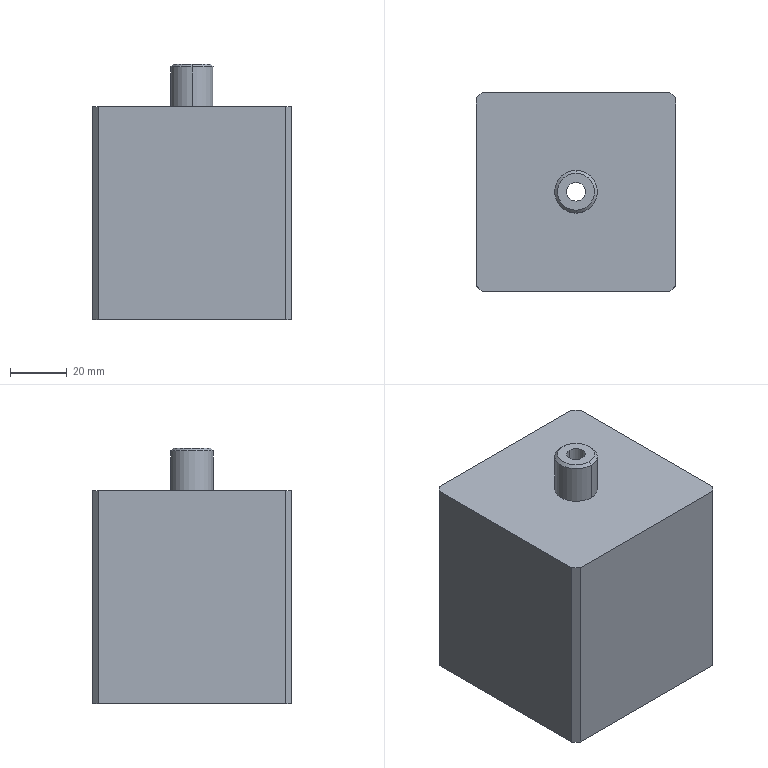NC program | NX | posted with a generic post | part box 70 x 70 x 90 mm
Lines 1 to 1715 of 2643, first 1589 of 1703 lines:
N10 G17 G21 G94 G90
(FLOOR_WALL , TOOL : D63)
N12 T01 M6
N14 G54
N16 G17 G0 G90 X-72.5 Y37.997 S6500 M3
N18 G43 Z30. H1
N20 Z3.
N22 G94 G1 Z0. F2500.
N24 X-69.5
N26 X69.5
N28 Y12.599
N30 X-69.5
N32 Y-12.8
N34 X69.5
N36 X72.5
N38 Z3.
N40 G0 Z30.
N42 M5
(DRILLING , TOOL : D8A45)
N44 T06 M6
N46 G54
N48 G17 G0 G90 X0. Y0. S5000 M3
N50 G43 Z30. H6
N52 G94 G81 G98 Z-3.4 F250. R3.
N54 G80
N56 G0 X0. Y0. Z30.
N58 M5
(DRILLING_COPY , TOOL : 6.6ZT)
N60 T16 M6
N62 G54
N64 G17 G0 G90 X0. Y0. S2000 M3
N66 G43 Z30. H16
N68 G94 G83 G98 Z-26.983 F250. Q2. R3.
N70 G80
N72 G0 X0. Y0. Z30.
N74 M5
(ZLEVEL_PROFILE , TOOL : D16)
N76 T22 M6
N78 G54
N80 G17 G0 G90 X-2.862 Y-43.15 S7500 M3
N82 G43 Z30. H22
N84 Z1.4
N86 G94 G1 X-33. Z-0.179 F1000.
N88 X-33.7 Z-0.216
N90 X-35.342 Y-42.838 Z-0.304
N92 X-36.886 Y-42.198 Z-0.391
N94 X-38.268 Y-41.258 Z-0.479
N96 X-41.258 Y-38.268 Z-0.701
N98 X-42.198 Y-36.886 Z-0.788
N100 X-42.838 Y-35.342 Z-0.876
N102 X-43.15 Y-33.7 Z-0.963
N104 Y-33. Z-1.
N106 Y33. F2500.
N108 G2 X-40.763 Y38.763 R8.15
N110 G1 X-38.763 Y40.763
N112 G2 X-33. Y43.15 R8.15
N114 G1 X33.
N116 G2 X38.763 Y40.763 R8.15
N118 G1 X40.763 Y38.763
N120 G2 X43.15 Y33. R8.15
N122 G1 Y-33.
N124 G2 X40.763 Y-38.763 R8.15
N126 G1 X38.763 Y-40.763
N128 G2 X33. Y-43.15 R8.15
N130 G1 X-33.
N132 G2 X-38.763 Y-40.763 R8.15
N134 G1 X-40.763 Y-38.763
N136 G2 X-43.15 Y-33. R8.15
N138 G1 Y24.29 Z-2.
N140 Y33.
N142 G2 X-40.763 Y38.763 R8.15
N144 G1 X-38.763 Y40.763
N146 G2 X-33. Y43.15 R8.15
N148 G1 X33.
N150 G2 X38.763 Y40.763 R8.15
N152 G1 X40.763 Y38.763
N154 G2 X43.15 Y33. R8.15
N156 G1 Y-33.
N158 G2 X40.763 Y-38.763 R8.15
N160 G1 X38.763 Y-40.763
N162 G2 X33. Y-43.15 R8.15
N164 G1 X-33.
N166 G2 X-38.763 Y-40.763 R8.15
N168 G1 X-40.763 Y-38.763
N170 G2 X-43.15 Y-33. R8.15
N172 G1 Y24.29 Z-3.
N174 Y33.
N176 G2 X-40.763 Y38.763 R8.15
N178 G1 X-38.763 Y40.763
N180 G2 X-33. Y43.15 R8.15
N182 G1 X33.
N184 G2 X38.763 Y40.763 R8.15
N186 G1 X40.763 Y38.763
N188 G2 X43.15 Y33. R8.15
N190 G1 Y-33.
N192 G2 X40.763 Y-38.763 R8.15
N194 G1 X38.763 Y-40.763
N196 G2 X33. Y-43.15 R8.15
N198 G1 X-33.
N200 G2 X-38.763 Y-40.763 R8.15
N202 G1 X-40.763 Y-38.763
N204 G2 X-43.15 Y-33. R8.15
N206 G1 Y24.29 Z-4.
N208 Y33.
N210 G2 X-40.763 Y38.763 R8.15
N212 G1 X-38.763 Y40.763
N214 G2 X-33. Y43.15 R8.15
N216 G1 X33.
N218 G2 X38.763 Y40.763 R8.15
N220 G1 X40.763 Y38.763
N222 G2 X43.15 Y33. R8.15
N224 G1 Y-33.
N226 G2 X40.763 Y-38.763 R8.15
N228 G1 X38.763 Y-40.763
N230 G2 X33. Y-43.15 R8.15
N232 G1 X-33.
N234 G2 X-38.763 Y-40.763 R8.15
N236 G1 X-40.763 Y-38.763
N238 G2 X-43.15 Y-33. R8.15
N240 G1 Y24.29 Z-5.
N242 Y33.
N244 G2 X-40.763 Y38.763 R8.15
N246 G1 X-38.763 Y40.763
N248 G2 X-33. Y43.15 R8.15
N250 G1 X33.
N252 G2 X38.763 Y40.763 R8.15
N254 G1 X40.763 Y38.763
N256 G2 X43.15 Y33. R8.15
N258 G1 Y-33.
N260 G2 X40.763 Y-38.763 R8.15
N262 G1 X38.763 Y-40.763
N264 G2 X33. Y-43.15 R8.15
N266 G1 X-33.
N268 G2 X-38.763 Y-40.763 R8.15
N270 G1 X-40.763 Y-38.763
N272 G2 X-43.15 Y-33. R8.15
N274 G1 Y24.29 Z-6.
N276 Y33.
N278 G2 X-40.763 Y38.763 R8.15
N280 G1 X-38.763 Y40.763
N282 G2 X-33. Y43.15 R8.15
N284 G1 X33.
N286 G2 X38.763 Y40.763 R8.15
N288 G1 X40.763 Y38.763
N290 G2 X43.15 Y33. R8.15
N292 G1 Y-33.
N294 G2 X40.763 Y-38.763 R8.15
N296 G1 X38.763 Y-40.763
N298 G2 X33. Y-43.15 R8.15
N300 G1 X-33.
N302 G2 X-38.763 Y-40.763 R8.15
N304 G1 X-40.763 Y-38.763
N306 G2 X-43.15 Y-33. R8.15
N308 G1 Y24.29 Z-7.
N310 Y33.
N312 G2 X-40.763 Y38.763 R8.15
N314 G1 X-38.763 Y40.763
N316 G2 X-33. Y43.15 R8.15
N318 G1 X33.
N320 G2 X38.763 Y40.763 R8.15
N322 G1 X40.763 Y38.763
N324 G2 X43.15 Y33. R8.15
N326 G1 Y-33.
N328 G2 X40.763 Y-38.763 R8.15
N330 G1 X38.763 Y-40.763
N332 G2 X33. Y-43.15 R8.15
N334 G1 X-33.
N336 G2 X-38.763 Y-40.763 R8.15
N338 G1 X-40.763 Y-38.763
N340 G2 X-43.15 Y-33. R8.15
N342 G1 Y24.29 Z-8.
N344 Y33.
N346 G2 X-40.763 Y38.763 R8.15
N348 G1 X-38.763 Y40.763
N350 G2 X-33. Y43.15 R8.15
N352 G1 X33.
N354 G2 X38.763 Y40.763 R8.15
N356 G1 X40.763 Y38.763
N358 G2 X43.15 Y33. R8.15
N360 G1 Y-33.
N362 G2 X40.763 Y-38.763 R8.15
N364 G1 X38.763 Y-40.763
N366 G2 X33. Y-43.15 R8.15
N368 G1 X-33.
N370 G2 X-38.763 Y-40.763 R8.15
N372 G1 X-40.763 Y-38.763
N374 G2 X-43.15 Y-33. R8.15
N376 G1 Y24.29 Z-9.
N378 Y33.
N380 G2 X-40.763 Y38.763 R8.15
N382 G1 X-38.763 Y40.763
N384 G2 X-33. Y43.15 R8.15
N386 G1 X33.
N388 G2 X38.763 Y40.763 R8.15
N390 G1 X40.763 Y38.763
N392 G2 X43.15 Y33. R8.15
N394 G1 Y-33.
N396 G2 X40.763 Y-38.763 R8.15
N398 G1 X38.763 Y-40.763
N400 G2 X33. Y-43.15 R8.15
N402 G1 X-33.
N404 G2 X-38.763 Y-40.763 R8.15
N406 G1 X-40.763 Y-38.763
N408 G2 X-43.15 Y-33. R8.15
N410 G1 Y24.29 Z-10.
N412 Y33.
N414 G2 X-40.763 Y38.763 R8.15
N416 G1 X-38.763 Y40.763
N418 G2 X-33. Y43.15 R8.15
N420 G1 X33.
N422 G2 X38.763 Y40.763 R8.15
N424 G1 X40.763 Y38.763
N426 G2 X43.15 Y33. R8.15
N428 G1 Y-33.
N430 G2 X40.763 Y-38.763 R8.15
N432 G1 X38.763 Y-40.763
N434 G2 X33. Y-43.15 R8.15
N436 G1 X-33.
N438 G2 X-38.763 Y-40.763 R8.15
N440 G1 X-40.763 Y-38.763
N442 G2 X-43.15 Y-33. R8.15
N444 G1 Y24.29 Z-11.
N446 Y33.
N448 G2 X-40.763 Y38.763 R8.15
N450 G1 X-38.763 Y40.763
N452 G2 X-33. Y43.15 R8.15
N454 G1 X33.
N456 G2 X38.763 Y40.763 R8.15
N458 G1 X40.763 Y38.763
N460 G2 X43.15 Y33. R8.15
N462 G1 Y-33.
N464 G2 X40.763 Y-38.763 R8.15
N466 G1 X38.763 Y-40.763
N468 G2 X33. Y-43.15 R8.15
N470 G1 X-33.
N472 G2 X-38.763 Y-40.763 R8.15
N474 G1 X-40.763 Y-38.763
N476 G2 X-43.15 Y-33. R8.15
N478 G1 Y24.29 Z-12.
N480 Y33.
N482 G2 X-40.763 Y38.763 R8.15
N484 G1 X-38.763 Y40.763
N486 G2 X-33. Y43.15 R8.15
N488 G1 X33.
N490 G2 X38.763 Y40.763 R8.15
N492 G1 X40.763 Y38.763
N494 G2 X43.15 Y33. R8.15
N496 G1 Y-33.
N498 G2 X40.763 Y-38.763 R8.15
N500 G1 X38.763 Y-40.763
N502 G2 X33. Y-43.15 R8.15
N504 G1 X-33.
N506 G2 X-38.763 Y-40.763 R8.15
N508 G1 X-40.763 Y-38.763
N510 G2 X-43.15 Y-33. R8.15
N512 G1 Y24.29 Z-13.
N514 Y33.
N516 G2 X-40.763 Y38.763 R8.15
N518 G1 X-38.763 Y40.763
N520 G2 X-33. Y43.15 R8.15
N522 G1 X33.
N524 G2 X38.763 Y40.763 R8.15
N526 G1 X40.763 Y38.763
N528 G2 X43.15 Y33. R8.15
N530 G1 Y-33.
N532 G2 X40.763 Y-38.763 R8.15
N534 G1 X38.763 Y-40.763
N536 G2 X33. Y-43.15 R8.15
N538 G1 X-33.
N540 G2 X-38.763 Y-40.763 R8.15
N542 G1 X-40.763 Y-38.763
N544 G2 X-43.15 Y-33. R8.15
N546 G1 Y24.29 Z-14.
N548 Y33.
N550 G2 X-40.763 Y38.763 R8.15
N552 G1 X-38.763 Y40.763
N554 G2 X-33. Y43.15 R8.15
N556 G1 X33.
N558 G2 X38.763 Y40.763 R8.15
N560 G1 X40.763 Y38.763
N562 G2 X43.15 Y33. R8.15
N564 G1 Y-33.
N566 G2 X40.763 Y-38.763 R8.15
N568 G1 X38.763 Y-40.763
N570 G2 X33. Y-43.15 R8.15
N572 G1 X-33.
N574 G2 X-38.763 Y-40.763 R8.15
N576 G1 X-40.763 Y-38.763
N578 G2 X-43.15 Y-33. R8.15
N580 G1 Y24.29 Z-15.
N582 Y33.
N584 G2 X-40.763 Y38.763 R8.15
N586 G1 X-38.763 Y40.763
N588 G2 X-33. Y43.15 R8.15
N590 G1 X33.
N592 G2 X38.763 Y40.763 R8.15
N594 G1 X40.763 Y38.763
N596 G2 X43.15 Y33. R8.15
N598 G1 Y-33.
N600 G2 X40.763 Y-38.763 R8.15
N602 G1 X38.763 Y-40.763
N604 G2 X33. Y-43.15 R8.15
N606 G1 X-33.
N608 G2 X-38.763 Y-40.763 R8.15
N610 G1 X-40.763 Y-38.763
N612 G2 X-43.15 Y-33. R8.15
N614 G1 Y24.29 Z-16.
N616 Y33.
N618 G2 X-40.763 Y38.763 R8.15
N620 G1 X-38.763 Y40.763
N622 G2 X-33. Y43.15 R8.15
N624 G1 X33.
N626 G2 X38.763 Y40.763 R8.15
N628 G1 X40.763 Y38.763
N630 G2 X43.15 Y33. R8.15
N632 G1 Y-33.
N634 G2 X40.763 Y-38.763 R8.15
N636 G1 X38.763 Y-40.763
N638 G2 X33. Y-43.15 R8.15
N640 G1 X-33.
N642 G2 X-38.763 Y-40.763 R8.15
N644 G1 X-40.763 Y-38.763
N646 G2 X-43.15 Y-33. R8.15
N648 G1 Y24.29 Z-17.
N650 Y33.
N652 G2 X-40.763 Y38.763 R8.15
N654 G1 X-38.763 Y40.763
N656 G2 X-33. Y43.15 R8.15
N658 G1 X33.
N660 G2 X38.763 Y40.763 R8.15
N662 G1 X40.763 Y38.763
N664 G2 X43.15 Y33. R8.15
N666 G1 Y-33.
N668 G2 X40.763 Y-38.763 R8.15
N670 G1 X38.763 Y-40.763
N672 G2 X33. Y-43.15 R8.15
N674 G1 X-33.
N676 G2 X-38.763 Y-40.763 R8.15
N678 G1 X-40.763 Y-38.763
N680 G2 X-43.15 Y-33. R8.15
N682 G1 Y24.29 Z-18.
N684 Y33.
N686 G2 X-40.763 Y38.763 R8.15
N688 G1 X-38.763 Y40.763
N690 G2 X-33. Y43.15 R8.15
N692 G1 X33.
N694 G2 X38.763 Y40.763 R8.15
N696 G1 X40.763 Y38.763
N698 G2 X43.15 Y33. R8.15
N700 G1 Y-33.
N702 G2 X40.763 Y-38.763 R8.15
N704 G1 X38.763 Y-40.763
N706 G2 X33. Y-43.15 R8.15
N708 G1 X-33.
N710 G2 X-38.763 Y-40.763 R8.15
N712 G1 X-40.763 Y-38.763
N714 G2 X-43.15 Y-33. R8.15
N716 G1 Y24.29 Z-19.
N718 Y33.
N720 G2 X-40.763 Y38.763 R8.15
N722 G1 X-38.763 Y40.763
N724 G2 X-33. Y43.15 R8.15
N726 G1 X33.
N728 G2 X38.763 Y40.763 R8.15
N730 G1 X40.763 Y38.763
N732 G2 X43.15 Y33. R8.15
N734 G1 Y-33.
N736 G2 X40.763 Y-38.763 R8.15
N738 G1 X38.763 Y-40.763
N740 G2 X33. Y-43.15 R8.15
N742 G1 X-33.
N744 G2 X-38.763 Y-40.763 R8.15
N746 G1 X-40.763 Y-38.763
N748 G2 X-43.15 Y-33. R8.15
N750 G1 Y24.29 Z-20.
N752 Y33.
N754 G2 X-40.763 Y38.763 R8.15
N756 G1 X-38.763 Y40.763
N758 G2 X-33. Y43.15 R8.15
N760 G1 X33.
N762 G2 X38.763 Y40.763 R8.15
N764 G1 X40.763 Y38.763
N766 G2 X43.15 Y33. R8.15
N768 G1 Y-33.
N770 G2 X40.763 Y-38.763 R8.15
N772 G1 X38.763 Y-40.763
N774 G2 X33. Y-43.15 R8.15
N776 G1 X-33.
N778 G2 X-38.763 Y-40.763 R8.15
N780 G1 X-40.763 Y-38.763
N782 G2 X-43.15 Y-33. R8.15
N784 G1 Y24.29 Z-21.
N786 Y33.
N788 G2 X-40.763 Y38.763 R8.15
N790 G1 X-38.763 Y40.763
N792 G2 X-33. Y43.15 R8.15
N794 G1 X33.
N796 G2 X38.763 Y40.763 R8.15
N798 G1 X40.763 Y38.763
N800 G2 X43.15 Y33. R8.15
N802 G1 Y-33.
N804 G2 X40.763 Y-38.763 R8.15
N806 G1 X38.763 Y-40.763
N808 G2 X33. Y-43.15 R8.15
N810 G1 X-33.
N812 G2 X-38.763 Y-40.763 R8.15
N814 G1 X-40.763 Y-38.763
N816 G2 X-43.15 Y-33. R8.15
N818 G1 Y24.29 Z-22.
N820 Y33.
N822 G2 X-40.763 Y38.763 R8.15
N824 G1 X-38.763 Y40.763
N826 G2 X-33. Y43.15 R8.15
N828 G1 X33.
N830 G2 X38.763 Y40.763 R8.15
N832 G1 X40.763 Y38.763
N834 G2 X43.15 Y33. R8.15
N836 G1 Y-33.
N838 G2 X40.763 Y-38.763 R8.15
N840 G1 X38.763 Y-40.763
N842 G2 X33. Y-43.15 R8.15
N844 G1 X-33.
N846 G2 X-38.763 Y-40.763 R8.15
N848 G1 X-40.763 Y-38.763
N850 G2 X-43.15 Y-33. R8.15
N852 G1 Y24.29 Z-23.
N854 Y33.
N856 G2 X-40.763 Y38.763 R8.15
N858 G1 X-38.763 Y40.763
N860 G2 X-33. Y43.15 R8.15
N862 G1 X33.
N864 G2 X38.763 Y40.763 R8.15
N866 G1 X40.763 Y38.763
N868 G2 X43.15 Y33. R8.15
N870 G1 Y-33.
N872 G2 X40.763 Y-38.763 R8.15
N874 G1 X38.763 Y-40.763
N876 G2 X33. Y-43.15 R8.15
N878 G1 X-33.
N880 G2 X-38.763 Y-40.763 R8.15
N882 G1 X-40.763 Y-38.763
N884 G2 X-43.15 Y-33. R8.15
N886 G1 Y24.29 Z-24.
N888 Y33.
N890 G2 X-40.763 Y38.763 R8.15
N892 G1 X-38.763 Y40.763
N894 G2 X-33. Y43.15 R8.15
N896 G1 X33.
N898 G2 X38.763 Y40.763 R8.15
N900 G1 X40.763 Y38.763
N902 G2 X43.15 Y33. R8.15
N904 G1 Y-33.
N906 G2 X40.763 Y-38.763 R8.15
N908 G1 X38.763 Y-40.763
N910 G2 X33. Y-43.15 R8.15
N912 G1 X-33.
N914 G2 X-38.763 Y-40.763 R8.15
N916 G1 X-40.763 Y-38.763
N918 G2 X-43.15 Y-33. R8.15
N920 G1 Y24.29 Z-25.
N922 Y33.
N924 G2 X-40.763 Y38.763 R8.15
N926 G1 X-38.763 Y40.763
N928 G2 X-33. Y43.15 R8.15
N930 G1 X33.
N932 G2 X38.763 Y40.763 R8.15
N934 G1 X40.763 Y38.763
N936 G2 X43.15 Y33. R8.15
N938 G1 Y-33.
N940 G2 X40.763 Y-38.763 R8.15
N942 G1 X38.763 Y-40.763
N944 G2 X33. Y-43.15 R8.15
N946 G1 X-33.
N948 G2 X-38.763 Y-40.763 R8.15
N950 G1 X-40.763 Y-38.763
N952 G2 X-43.15 Y-33. R8.15
N954 G1 Y24.29 Z-26.
N956 Y33.
N958 G2 X-40.763 Y38.763 R8.15
N960 G1 X-38.763 Y40.763
N962 G2 X-33. Y43.15 R8.15
N964 G1 X33.
N966 G2 X38.763 Y40.763 R8.15
N968 G1 X40.763 Y38.763
N970 G2 X43.15 Y33. R8.15
N972 G1 Y-33.
N974 G2 X40.763 Y-38.763 R8.15
N976 G1 X38.763 Y-40.763
N978 G2 X33. Y-43.15 R8.15
N980 G1 X-33.
N982 G2 X-38.763 Y-40.763 R8.15
N984 G1 X-40.763 Y-38.763
N986 G2 X-43.15 Y-33. R8.15
N988 G1 Y24.29 Z-27.
N990 Y33.
N992 G2 X-40.763 Y38.763 R8.15
N994 G1 X-38.763 Y40.763
N996 G2 X-33. Y43.15 R8.15
N998 G1 X33.
N1000 G2 X38.763 Y40.763 R8.15
N1002 G1 X40.763 Y38.763
N1004 G2 X43.15 Y33. R8.15
N1006 G1 Y-33.
N1008 G2 X40.763 Y-38.763 R8.15
N1010 G1 X38.763 Y-40.763
N1012 G2 X33. Y-43.15 R8.15
N1014 G1 X-33.
N1016 G2 X-38.763 Y-40.763 R8.15
N1018 G1 X-40.763 Y-38.763
N1020 G2 X-43.15 Y-33. R8.15
N1022 G1 Y24.29 Z-28.
N1024 Y33.
N1026 G2 X-40.763 Y38.763 R8.15
N1028 G1 X-38.763 Y40.763
N1030 G2 X-33. Y43.15 R8.15
N1032 G1 X33.
N1034 G2 X38.763 Y40.763 R8.15
N1036 G1 X40.763 Y38.763
N1038 G2 X43.15 Y33. R8.15
N1040 G1 Y-33.
N1042 G2 X40.763 Y-38.763 R8.15
N1044 G1 X38.763 Y-40.763
N1046 G2 X33. Y-43.15 R8.15
N1048 G1 X-33.
N1050 G2 X-38.763 Y-40.763 R8.15
N1052 G1 X-40.763 Y-38.763
N1054 G2 X-43.15 Y-33. R8.15
N1056 G1 Y24.29 Z-29.
N1058 Y33.
N1060 G2 X-40.763 Y38.763 R8.15
N1062 G1 X-38.763 Y40.763
N1064 G2 X-33. Y43.15 R8.15
N1066 G1 X33.
N1068 G2 X38.763 Y40.763 R8.15
N1070 G1 X40.763 Y38.763
N1072 G2 X43.15 Y33. R8.15
N1074 G1 Y-33.
N1076 G2 X40.763 Y-38.763 R8.15
N1078 G1 X38.763 Y-40.763
N1080 G2 X33. Y-43.15 R8.15
N1082 G1 X-33.
N1084 G2 X-38.763 Y-40.763 R8.15
N1086 G1 X-40.763 Y-38.763
N1088 G2 X-43.15 Y-33. R8.15
N1090 G1 Y24.29 Z-30.
N1092 Y33.
N1094 G2 X-40.763 Y38.763 R8.15
N1096 G1 X-38.763 Y40.763
N1098 G2 X-33. Y43.15 R8.15
N1100 G1 X33.
N1102 G2 X38.763 Y40.763 R8.15
N1104 G1 X40.763 Y38.763
N1106 G2 X43.15 Y33. R8.15
N1108 G1 Y-33.
N1110 G2 X40.763 Y-38.763 R8.15
N1112 G1 X38.763 Y-40.763
N1114 G2 X33. Y-43.15 R8.15
N1116 G1 X-33.
N1118 G2 X-38.763 Y-40.763 R8.15
N1120 G1 X-40.763 Y-38.763
N1122 G2 X-43.15 Y-33. R8.15
N1124 G1 Y24.29 Z-31.
N1126 Y33.
N1128 G2 X-40.763 Y38.763 R8.15
N1130 G1 X-38.763 Y40.763
N1132 G2 X-33. Y43.15 R8.15
N1134 G1 X33.
N1136 G2 X38.763 Y40.763 R8.15
N1138 G1 X40.763 Y38.763
N1140 G2 X43.15 Y33. R8.15
N1142 G1 Y-33.
N1144 G2 X40.763 Y-38.763 R8.15
N1146 G1 X38.763 Y-40.763
N1148 G2 X33. Y-43.15 R8.15
N1150 G1 X-33.
N1152 G2 X-38.763 Y-40.763 R8.15
N1154 G1 X-40.763 Y-38.763
N1156 G2 X-43.15 Y-33. R8.15
N1158 G1 Y24.29 Z-32.
N1160 Y33.
N1162 G2 X-40.763 Y38.763 R8.15
N1164 G1 X-38.763 Y40.763
N1166 G2 X-33. Y43.15 R8.15
N1168 G1 X33.
N1170 G2 X38.763 Y40.763 R8.15
N1172 G1 X40.763 Y38.763
N1174 G2 X43.15 Y33. R8.15
N1176 G1 Y-33.
N1178 G2 X40.763 Y-38.763 R8.15
N1180 G1 X38.763 Y-40.763
N1182 G2 X33. Y-43.15 R8.15
N1184 G1 X-33.
N1186 G2 X-38.763 Y-40.763 R8.15
N1188 G1 X-40.763 Y-38.763
N1190 G2 X-43.15 Y-33. R8.15
N1192 G1 Y24.29 Z-33.
N1194 Y33.
N1196 G2 X-40.763 Y38.763 R8.15
N1198 G1 X-38.763 Y40.763
N1200 G2 X-33. Y43.15 R8.15
N1202 G1 X33.
N1204 G2 X38.763 Y40.763 R8.15
N1206 G1 X40.763 Y38.763
N1208 G2 X43.15 Y33. R8.15
N1210 G1 Y-33.
N1212 G2 X40.763 Y-38.763 R8.15
N1214 G1 X38.763 Y-40.763
N1216 G2 X33. Y-43.15 R8.15
N1218 G1 X-33.
N1220 G2 X-38.763 Y-40.763 R8.15
N1222 G1 X-40.763 Y-38.763
N1224 G2 X-43.15 Y-33. R8.15
N1226 G1 Y24.29 Z-34.
N1228 Y33.
N1230 G2 X-40.763 Y38.763 R8.15
N1232 G1 X-38.763 Y40.763
N1234 G2 X-33. Y43.15 R8.15
N1236 G1 X33.
N1238 G2 X38.763 Y40.763 R8.15
N1240 G1 X40.763 Y38.763
N1242 G2 X43.15 Y33. R8.15
N1244 G1 Y-33.
N1246 G2 X40.763 Y-38.763 R8.15
N1248 G1 X38.763 Y-40.763
N1250 G2 X33. Y-43.15 R8.15
N1252 G1 X-33.
N1254 G2 X-38.763 Y-40.763 R8.15
N1256 G1 X-40.763 Y-38.763
N1258 G2 X-43.15 Y-33. R8.15
N1260 G1 Y24.29 Z-35.
N1262 Y33.
N1264 G2 X-40.763 Y38.763 R8.15
N1266 G1 X-38.763 Y40.763
N1268 G2 X-33. Y43.15 R8.15
N1270 G1 X33.
N1272 G2 X38.763 Y40.763 R8.15
N1274 G1 X40.763 Y38.763
N1276 G2 X43.15 Y33. R8.15
N1278 G1 Y-33.
N1280 G2 X40.763 Y-38.763 R8.15
N1282 G1 X38.763 Y-40.763
N1284 G2 X33. Y-43.15 R8.15
N1286 G1 X-33.
N1288 G2 X-38.763 Y-40.763 R8.15
N1290 G1 X-40.763 Y-38.763
N1292 G2 X-43.15 Y-33. R8.15
N1294 G1 Y24.29 Z-36.
N1296 Y33.
N1298 G2 X-40.763 Y38.763 R8.15
N1300 G1 X-38.763 Y40.763
N1302 G2 X-33. Y43.15 R8.15
N1304 G1 X33.
N1306 G2 X38.763 Y40.763 R8.15
N1308 G1 X40.763 Y38.763
N1310 G2 X43.15 Y33. R8.15
N1312 G1 Y-33.
N1314 G2 X40.763 Y-38.763 R8.15
N1316 G1 X38.763 Y-40.763
N1318 G2 X33. Y-43.15 R8.15
N1320 G1 X-33.
N1322 G2 X-38.763 Y-40.763 R8.15
N1324 G1 X-40.763 Y-38.763
N1326 G2 X-43.15 Y-33. R8.15
N1328 G1 Y24.29 Z-37.
N1330 Y33.
N1332 G2 X-40.763 Y38.763 R8.15
N1334 G1 X-38.763 Y40.763
N1336 G2 X-33. Y43.15 R8.15
N1338 G1 X33.
N1340 G2 X38.763 Y40.763 R8.15
N1342 G1 X40.763 Y38.763
N1344 G2 X43.15 Y33. R8.15
N1346 G1 Y-33.
N1348 G2 X40.763 Y-38.763 R8.15
N1350 G1 X38.763 Y-40.763
N1352 G2 X33. Y-43.15 R8.15
N1354 G1 X-33.
N1356 G2 X-38.763 Y-40.763 R8.15
N1358 G1 X-40.763 Y-38.763
N1360 G2 X-43.15 Y-33. R8.15
N1362 G1 Y24.29 Z-38.
N1364 Y33.
N1366 G2 X-40.763 Y38.763 R8.15
N1368 G1 X-38.763 Y40.763
N1370 G2 X-33. Y43.15 R8.15
N1372 G1 X33.
N1374 G2 X38.763 Y40.763 R8.15
N1376 G1 X40.763 Y38.763
N1378 G2 X43.15 Y33. R8.15
N1380 G1 Y-33.
N1382 G2 X40.763 Y-38.763 R8.15
N1384 G1 X38.763 Y-40.763
N1386 G2 X33. Y-43.15 R8.15
N1388 G1 X-33.
N1390 G2 X-38.763 Y-40.763 R8.15
N1392 G1 X-40.763 Y-38.763
N1394 G2 X-43.15 Y-33. R8.15
N1396 G1 Y24.29 Z-39.
N1398 Y33.
N1400 G2 X-40.763 Y38.763 R8.15
N1402 G1 X-38.763 Y40.763
N1404 G2 X-33. Y43.15 R8.15
N1406 G1 X33.
N1408 G2 X38.763 Y40.763 R8.15
N1410 G1 X40.763 Y38.763
N1412 G2 X43.15 Y33. R8.15
N1414 G1 Y-33.
N1416 G2 X40.763 Y-38.763 R8.15
N1418 G1 X38.763 Y-40.763
N1420 G2 X33. Y-43.15 R8.15
N1422 G1 X-33.
N1424 G2 X-38.763 Y-40.763 R8.15
N1426 G1 X-40.763 Y-38.763
N1428 G2 X-43.15 Y-33. R8.15
N1430 G1 Y24.29 Z-40.
N1432 Y33.
N1434 G2 X-40.763 Y38.763 R8.15
N1436 G1 X-38.763 Y40.763
N1438 G2 X-33. Y43.15 R8.15
N1440 G1 X33.
N1442 G2 X38.763 Y40.763 R8.15
N1444 G1 X40.763 Y38.763
N1446 G2 X43.15 Y33. R8.15
N1448 G1 Y-33.
N1450 G2 X40.763 Y-38.763 R8.15
N1452 G1 X38.763 Y-40.763
N1454 G2 X33. Y-43.15 R8.15
N1456 G1 X-33.
N1458 G2 X-38.763 Y-40.763 R8.15
N1460 G1 X-40.763 Y-38.763
N1462 G2 X-43.15 Y-33. R8.15
N1464 G1 Y24.29 Z-41.
N1466 Y33.
N1468 G2 X-40.763 Y38.763 R8.15
N1470 G1 X-38.763 Y40.763
N1472 G2 X-33. Y43.15 R8.15
N1474 G1 X33.
N1476 G2 X38.763 Y40.763 R8.15
N1478 G1 X40.763 Y38.763
N1480 G2 X43.15 Y33. R8.15
N1482 G1 Y-33.
N1484 G2 X40.763 Y-38.763 R8.15
N1486 G1 X38.763 Y-40.763
N1488 G2 X33. Y-43.15 R8.15
N1490 G1 X-33.
N1492 G2 X-38.763 Y-40.763 R8.15
N1494 G1 X-40.763 Y-38.763
N1496 G2 X-43.15 Y-33. R8.15
N1498 G1 Y24.29 Z-42.
N1500 Y33.
N1502 G2 X-40.763 Y38.763 R8.15
N1504 G1 X-38.763 Y40.763
N1506 G2 X-33. Y43.15 R8.15
N1508 G1 X33.
N1510 G2 X38.763 Y40.763 R8.15
N1512 G1 X40.763 Y38.763
N1514 G2 X43.15 Y33. R8.15
N1516 G1 Y-33.
N1518 G2 X40.763 Y-38.763 R8.15
N1520 G1 X38.763 Y-40.763
N1522 G2 X33. Y-43.15 R8.15
N1524 G1 X-33.
N1526 G2 X-38.763 Y-40.763 R8.15
N1528 G1 X-40.763 Y-38.763
N1530 G2 X-43.15 Y-33. R8.15
N1532 G1 Y24.29 Z-43.
N1534 Y33.
N1536 G2 X-40.763 Y38.763 R8.15
N1538 G1 X-38.763 Y40.763
N1540 G2 X-33. Y43.15 R8.15
N1542 G1 X33.
N1544 G2 X38.763 Y40.763 R8.15
N1546 G1 X40.763 Y38.763
N1548 G2 X43.15 Y33. R8.15
N1550 G1 Y-33.
N1552 G2 X40.763 Y-38.763 R8.15
N1554 G1 X38.763 Y-40.763
N1556 G2 X33. Y-43.15 R8.15
N1558 G1 X-33.
N1560 G2 X-38.763 Y-40.763 R8.15
N1562 G1 X-40.763 Y-38.763
N1564 G2 X-43.15 Y-33. R8.15
N1566 G1 Y24.29 Z-44.
N1568 Y33.
N1570 G2 X-40.763 Y38.763 R8.15
N1572 G1 X-38.763 Y40.763
N1574 G2 X-33. Y43.15 R8.15
N1576 G1 X33.
N1578 G2 X38.763 Y40.763 R8.15
N1580 G1 X40.763 Y38.763
N1582 G2 X43.15 Y33. R8.15
N1584 G1 Y-33.
N1586 G2 X40.763 Y-38.763 R8.15
N1588 G1 X38.763 Y-40.763
N1590 G2 X33. Y-43.15 R8.15
N1592 G1 X-33.
N1594 G2 X-38.763 Y-40.763 R8.15
N1596 G1 X-40.763 Y-38.763
N1598 G2 X-43.15 Y-33. R8.15
N1600 G1 Y24.29 Z-45.
N1602 Y33.
N1604 G2 X-40.763 Y38.763 R8.15
N1606 G1 X-38.763 Y40.763
N1608 G2 X-33. Y43.15 R8.15
N1610 G1 X33.
N1612 G2 X38.763 Y40.763 R8.15
N1614 G1 X40.763 Y38.763
N1616 G2 X43.15 Y33. R8.15
N1618 G1 Y-33.
N1620 G2 X40.763 Y-38.763 R8.15
N1622 G1 X38.763 Y-40.763
N1624 G2 X33. Y-43.15 R8.15
N1626 G1 X-33.
N1628 G2 X-38.763 Y-40.763 R8.15
N1630 G1 X-40.763 Y-38.763
N1632 G2 X-43.15 Y-33. R8.15
N1634 G1 Y24.29 Z-46.
N1636 Y33.
N1638 G2 X-40.763 Y38.763 R8.15
N1640 G1 X-38.763 Y40.763
N1642 G2 X-33. Y43.15 R8.15
N1644 G1 X33.
N1646 G2 X38.763 Y40.763 R8.15
N1648 G1 X40.763 Y38.763
N1650 G2 X43.15 Y33. R8.15
N1652 G1 Y-33.
N1654 G2 X40.763 Y-38.763 R8.15
N1656 G1 X38.763 Y-40.763
N1658 G2 X33. Y-43.15 R8.15
N1660 G1 X-33.
N1662 G2 X-38.763 Y-40.763 R8.15
N1664 G1 X-40.763 Y-38.763
N1666 G2 X-43.15 Y-33. R8.15
N1668 G1 Y24.29 Z-47.
N1670 Y33.
N1672 G2 X-40.763 Y38.763 R8.15
N1674 G1 X-38.763 Y40.763
N1676 G2 X-33. Y43.15 R8.15
N1678 G1 X33.
N1680 G2 X38.763 Y40.763 R8.15
N1682 G1 X40.763 Y38.763
N1684 G2 X43.15 Y33. R8.15
N1686 G1 Y-33.
N1688 G2 X40.763 Y-38.763 R8.15
N1690 G1 X38.763 Y-40.763
N1692 G2 X33. Y-43.15 R8.15
N1694 G1 X-33.
N1696 G2 X-38.763 Y-40.763 R8.15
N1698 G1 X-40.763 Y-38.763
N1700 G2 X-43.15 Y-33. R8.15
N1702 G1 Y24.29 Z-48.
N1704 Y33.
N1706 G2 X-40.763 Y38.763 R8.15
N1708 G1 X-38.763 Y40.763
N1710 G2 X-33. Y43.15 R8.15
N1712 G1 X33.
N1714 G2 X38.763 Y40.763 R8.15
N1716 G1 X40.763 Y38.763
N1718 G2 X43.15 Y33. R8.15
N1720 G1 Y-33.
N1722 G2 X40.763 Y-38.763 R8.15
N1724 G1 X38.763 Y-40.763
N1726 G2 X33. Y-43.15 R8.15
N1728 G1 X-33.
N1730 G2 X-38.763 Y-40.763 R8.15
N1732 G1 X-40.763 Y-38.763
N1734 G2 X-43.15 Y-33. R8.15
N1736 G1 Y24.29 Z-49.
N1738 Y33.
N1740 G2 X-40.763 Y38.763 R8.15
N1742 G1 X-38.763 Y40.763
N1744 G2 X-33. Y43.15 R8.15
N1746 G1 X33.
N1748 G2 X38.763 Y40.763 R8.15
N1750 G1 X40.763 Y38.763
N1752 G2 X43.15 Y33. R8.15
N1754 G1 Y-33.
N1756 G2 X40.763 Y-38.763 R8.15
N1758 G1 X38.763 Y-40.763
N1760 G2 X33. Y-43.15 R8.15
N1762 G1 X-33.
N1764 G2 X-38.763 Y-40.763 R8.15
N1766 G1 X-40.763 Y-38.763
N1768 G2 X-43.15 Y-33. R8.15
N1770 G1 Y24.29 Z-50.
N1772 Y33.
N1774 G2 X-40.763 Y38.763 R8.15
N1776 G1 X-38.763 Y40.763
N1778 G2 X-33. Y43.15 R8.15
N1780 G1 X33.
N1782 G2 X38.763 Y40.763 R8.15
N1784 G1 X40.763 Y38.763
N1786 G2 X43.15 Y33. R8.15
N1788 G1 Y-33.
N1790 G2 X40.763 Y-38.763 R8.15
N1792 G1 X38.763 Y-40.763
N1794 G2 X33. Y-43.15 R8.15
N1796 G1 X-33.
N1798 G2 X-38.763 Y-40.763 R8.15
N1800 G1 X-40.763 Y-38.763
N1802 G2 X-43.15 Y-33. R8.15
N1804 G1 Y24.29 Z-51.
N1806 Y33.
N1808 G2 X-40.763 Y38.763 R8.15
N1810 G1 X-38.763 Y40.763
N1812 G2 X-33. Y43.15 R8.15
N1814 G1 X33.
N1816 G2 X38.763 Y40.763 R8.15
N1818 G1 X40.763 Y38.763
N1820 G2 X43.15 Y33. R8.15
N1822 G1 Y-33.
N1824 G2 X40.763 Y-38.763 R8.15
N1826 G1 X38.763 Y-40.763
N1828 G2 X33. Y-43.15 R8.15
N1830 G1 X-33.
N1832 G2 X-38.763 Y-40.763 R8.15
N1834 G1 X-40.763 Y-38.763
N1836 G2 X-43.15 Y-33. R8.15
N1838 G1 Y24.29 Z-52.
N1840 Y33.
N1842 G2 X-40.763 Y38.763 R8.15
N1844 G1 X-38.763 Y40.763
N1846 G2 X-33. Y43.15 R8.15
N1848 G1 X33.
N1850 G2 X38.763 Y40.763 R8.15
N1852 G1 X40.763 Y38.763
N1854 G2 X43.15 Y33. R8.15
N1856 G1 Y-33.
N1858 G2 X40.763 Y-38.763 R8.15
N1860 G1 X38.763 Y-40.763
N1862 G2 X33. Y-43.15 R8.15
N1864 G1 X-33.
N1866 G2 X-38.763 Y-40.763 R8.15
N1868 G1 X-40.763 Y-38.763
N1870 G2 X-43.15 Y-33. R8.15
N1872 G1 Y24.29 Z-53.
N1874 Y33.
N1876 G2 X-40.763 Y38.763 R8.15
N1878 G1 X-38.763 Y40.763
N1880 G2 X-33. Y43.15 R8.15
N1882 G1 X33.
N1884 G2 X38.763 Y40.763 R8.15
N1886 G1 X40.763 Y38.763
N1888 G2 X43.15 Y33. R8.15
N1890 G1 Y-33.
N1892 G2 X40.763 Y-38.763 R8.15
N1894 G1 X38.763 Y-40.763
N1896 G2 X33. Y-43.15 R8.15
N1898 G1 X-33.
N1900 G2 X-38.763 Y-40.763 R8.15
N1902 G1 X-40.763 Y-38.763
N1904 G2 X-43.15 Y-33. R8.15
N1906 G1 Y24.29 Z-54.
N1908 Y33.
N1910 G2 X-40.763 Y38.763 R8.15
N1912 G1 X-38.763 Y40.763
N1914 G2 X-33. Y43.15 R8.15
N1916 G1 X33.
N1918 G2 X38.763 Y40.763 R8.15
N1920 G1 X40.763 Y38.763
N1922 G2 X43.15 Y33. R8.15
N1924 G1 Y-33.
N1926 G2 X40.763 Y-38.763 R8.15
N1928 G1 X38.763 Y-40.763
N1930 G2 X33. Y-43.15 R8.15
N1932 G1 X-33.
N1934 G2 X-38.763 Y-40.763 R8.15
N1936 G1 X-40.763 Y-38.763
N1938 G2 X-43.15 Y-33. R8.15
N1940 G1 Y24.29 Z-55.
N1942 Y33.
N1944 G2 X-40.763 Y38.763 R8.15
N1946 G1 X-38.763 Y40.763
N1948 G2 X-33. Y43.15 R8.15
N1950 G1 X33.
N1952 G2 X38.763 Y40.763 R8.15
N1954 G1 X40.763 Y38.763
N1956 G2 X43.15 Y33. R8.15
N1958 G1 Y-33.
N1960 G2 X40.763 Y-38.763 R8.15
N1962 G1 X38.763 Y-40.763
N1964 G2 X33. Y-43.15 R8.15
N1966 G1 X-33.
N1968 G2 X-38.763 Y-40.763 R8.15
N1970 G1 X-40.763 Y-38.763
N1972 G2 X-43.15 Y-33. R8.15
N1974 G1 Y24.29 Z-56.
N1976 Y33.
N1978 G2 X-40.763 Y38.763 R8.15
N1980 G1 X-38.763 Y40.763
N1982 G2 X-33. Y43.15 R8.15
N1984 G1 X33.
N1986 G2 X38.763 Y40.763 R8.15
N1988 G1 X40.763 Y38.763
N1990 G2 X43.15 Y33. R8.15
N1992 G1 Y-33.
N1994 G2 X40.763 Y-38.763 R8.15
N1996 G1 X38.763 Y-40.763
N1998 G2 X33. Y-43.15 R8.15
N2000 G1 X-33.
N2002 G2 X-38.763 Y-40.763 R8.15
N2004 G1 X-40.763 Y-38.763
N2006 G2 X-43.15 Y-33. R8.15
N2008 G1 Y24.29 Z-57.
N2010 Y33.
N2012 G2 X-40.763 Y38.763 R8.15
N2014 G1 X-38.763 Y40.763
N2016 G2 X-33. Y43.15 R8.15
N2018 G1 X33.
N2020 G2 X38.763 Y40.763 R8.15
N2022 G1 X40.763 Y38.763
N2024 G2 X43.15 Y33. R8.15
N2026 G1 Y-33.
N2028 G2 X40.763 Y-38.763 R8.15
N2030 G1 X38.763 Y-40.763
N2032 G2 X33. Y-43.15 R8.15
N2034 G1 X-33.
N2036 G2 X-38.763 Y-40.763 R8.15
N2038 G1 X-40.763 Y-38.763
N2040 G2 X-43.15 Y-33. R8.15
N2042 G1 Y24.29 Z-58.
N2044 Y33.
N2046 G2 X-40.763 Y38.763 R8.15
N2048 G1 X-38.763 Y40.763
N2050 G2 X-33. Y43.15 R8.15
N2052 G1 X33.
N2054 G2 X38.763 Y40.763 R8.15
N2056 G1 X40.763 Y38.763
N2058 G2 X43.15 Y33. R8.15
N2060 G1 Y-33.
N2062 G2 X40.763 Y-38.763 R8.15
N2064 G1 X38.763 Y-40.763
N2066 G2 X33. Y-43.15 R8.15
N2068 G1 X-33.
N2070 G2 X-38.763 Y-40.763 R8.15
N2072 G1 X-40.763 Y-38.763
N2074 G2 X-43.15 Y-33. R8.15
N2076 G1 Y24.29 Z-59.
N2078 Y33.
N2080 G2 X-40.763 Y38.763 R8.15
N2082 G1 X-38.763 Y40.763
N2084 G2 X-33. Y43.15 R8.15
N2086 G1 X33.
N2088 G2 X38.763 Y40.763 R8.15
N2090 G1 X40.763 Y38.763
N2092 G2 X43.15 Y33. R8.15
N2094 G1 Y-33.
N2096 G2 X40.763 Y-38.763 R8.15
N2098 G1 X38.763 Y-40.763
N2100 G2 X33. Y-43.15 R8.15
N2102 G1 X-33.
N2104 G2 X-38.763 Y-40.763 R8.15
N2106 G1 X-40.763 Y-38.763
N2108 G2 X-43.15 Y-33. R8.15
N2110 G1 Y24.29 Z-60.
N2112 Y33.
N2114 G2 X-40.763 Y38.763 R8.15
N2116 G1 X-38.763 Y40.763
N2118 G2 X-33. Y43.15 R8.15
N2120 G1 X33.
N2122 G2 X38.763 Y40.763 R8.15
N2124 G1 X40.763 Y38.763
N2126 G2 X43.15 Y33. R8.15
N2128 G1 Y-33.
N2130 G2 X40.763 Y-38.763 R8.15
N2132 G1 X38.763 Y-40.763
N2134 G2 X33. Y-43.15 R8.15
N2136 G1 X-33.
N2138 G2 X-38.763 Y-40.763 R8.15
N2140 G1 X-40.763 Y-38.763
N2142 G2 X-43.15 Y-33. R8.15
N2144 G1 Y24.29 Z-61.
N2146 Y33.
N2148 G2 X-40.763 Y38.763 R8.15
N2150 G1 X-38.763 Y40.763
N2152 G2 X-33. Y43.15 R8.15
N2154 G1 X33.
N2156 G2 X38.763 Y40.763 R8.15
N2158 G1 X40.763 Y38.763
N2160 G2 X43.15 Y33. R8.15
N2162 G1 Y-33.
N2164 G2 X40.763 Y-38.763 R8.15
N2166 G1 X38.763 Y-40.763
N2168 G2 X33. Y-43.15 R8.15
N2170 G1 X-33.
N2172 G2 X-38.763 Y-40.763 R8.15
N2174 G1 X-40.763 Y-38.763
N2176 G2 X-43.15 Y-33. R8.15
N2178 G1 Y24.29 Z-62.
N2180 Y33.
N2182 G2 X-40.763 Y38.763 R8.15
N2184 G1 X-38.763 Y40.763
N2186 G2 X-33. Y43.15 R8.15
N2188 G1 X33.
N2190 G2 X38.763 Y40.763 R8.15
N2192 G1 X40.763 Y38.763
N2194 G2 X43.15 Y33. R8.15
N2196 G1 Y-33.
N2198 G2 X40.763 Y-38.763 R8.15
N2200 G1 X38.763 Y-40.763
N2202 G2 X33. Y-43.15 R8.15
N2204 G1 X-33.
N2206 G2 X-38.763 Y-40.763 R8.15
N2208 G1 X-40.763 Y-38.763
N2210 G2 X-43.15 Y-33. R8.15
N2212 G1 Y24.29 Z-63.
N2214 Y33.
N2216 G2 X-40.763 Y38.763 R8.15
N2218 G1 X-38.763 Y40.763
N2220 G2 X-33. Y43.15 R8.15
N2222 G1 X33.
N2224 G2 X38.763 Y40.763 R8.15
N2226 G1 X40.763 Y38.763
N2228 G2 X43.15 Y33. R8.15
N2230 G1 Y-33.
N2232 G2 X40.763 Y-38.763 R8.15
N2234 G1 X38.763 Y-40.763
N2236 G2 X33. Y-43.15 R8.15
N2238 G1 X-33.
N2240 G2 X-38.763 Y-40.763 R8.15
N2242 G1 X-40.763 Y-38.763
N2244 G2 X-43.15 Y-33. R8.15
N2246 G1 Y24.29 Z-64.
N2248 Y33.
N2250 G2 X-40.763 Y38.763 R8.15
N2252 G1 X-38.763 Y40.763
N2254 G2 X-33. Y43.15 R8.15
N2256 G1 X33.
N2258 G2 X38.763 Y40.763 R8.15
N2260 G1 X40.763 Y38.763
N2262 G2 X43.15 Y33. R8.15
N2264 G1 Y-33.
N2266 G2 X40.763 Y-38.763 R8.15
N2268 G1 X38.763 Y-40.763
N2270 G2 X33. Y-43.15 R8.15
N2272 G1 X-33.
N2274 G2 X-38.763 Y-40.763 R8.15
N2276 G1 X-40.763 Y-38.763
N2278 G2 X-43.15 Y-33. R8.15
N2280 G1 Y24.29 Z-65.
N2282 Y33.
N2284 G2 X-40.763 Y38.763 R8.15
N2286 G1 X-38.763 Y40.763
N2288 G2 X-33. Y43.15 R8.15
N2290 G1 X33.
N2292 G2 X38.763 Y40.763 R8.15
N2294 G1 X40.763 Y38.763
N2296 G2 X43.15 Y33. R8.15
N2298 G1 Y-33.
N2300 G2 X40.763 Y-38.763 R8.15
N2302 G1 X38.763 Y-40.763
N2304 G2 X33. Y-43.15 R8.15
N2306 G1 X-33.
N2308 G2 X-38.763 Y-40.763 R8.15
N2310 G1 X-40.763 Y-38.763
N2312 G2 X-43.15 Y-33. R8.15
N2314 G1 Y24.29 Z-66.
N2316 Y33.
N2318 G2 X-40.763 Y38.763 R8.15
N2320 G1 X-38.763 Y40.763
N2322 G2 X-33. Y43.15 R8.15
N2324 G1 X33.
N2326 G2 X38.763 Y40.763 R8.15
N2328 G1 X40.763 Y38.763
N2330 G2 X43.15 Y33. R8.15
N2332 G1 Y-33.
N2334 G2 X40.763 Y-38.763 R8.15
N2336 G1 X38.763 Y-40.763
N2338 G2 X33. Y-43.15 R8.15
N2340 G1 X-33.
N2342 G2 X-38.763 Y-40.763 R8.15
N2344 G1 X-40.763 Y-38.763
N2346 G2 X-43.15 Y-33. R8.15
N2348 G1 Y24.29 Z-67.
N2350 Y33.
N2352 G2 X-40.763 Y38.763 R8.15
N2354 G1 X-38.763 Y40.763
N2356 G2 X-33. Y43.15 R8.15
N2358 G1 X33.
N2360 G2 X38.763 Y40.763 R8.15
N2362 G1 X40.763 Y38.763
N2364 G2 X43.15 Y33. R8.15
N2366 G1 Y-33.
N2368 G2 X40.763 Y-38.763 R8.15
N2370 G1 X38.763 Y-40.763
N2372 G2 X33. Y-43.15 R8.15
N2374 G1 X-33.
N2376 G2 X-38.763 Y-40.763 R8.15
N2378 G1 X-40.763 Y-38.763
N2380 G2 X-43.15 Y-33. R8.15
N2382 G1 Y24.29 Z-68.
N2384 Y33.
N2386 G2 X-40.763 Y38.763 R8.15
N2388 G1 X-38.763 Y40.763
N2390 G2 X-33. Y43.15 R8.15
N2392 G1 X33.
N2394 G2 X38.763 Y40.763 R8.15
N2396 G1 X40.763 Y38.763
N2398 G2 X43.15 Y33. R8.15
N2400 G1 Y-33.
N2402 G2 X40.763 Y-38.763 R8.15
N2404 G1 X38.763 Y-40.763
N2406 G2 X33. Y-43.15 R8.15
N2408 G1 X-33.
N2410 G2 X-38.763 Y-40.763 R8.15
N2412 G1 X-40.763 Y-38.763
N2414 G2 X-43.15 Y-33. R8.15
N2416 G1 Y24.29 Z-69.
N2418 Y33.
N2420 G2 X-40.763 Y38.763 R8.15
N2422 G1 X-38.763 Y40.763
N2424 G2 X-33. Y43.15 R8.15
N2426 G1 X33.
N2428 G2 X38.763 Y40.763 R8.15
N2430 G1 X40.763 Y38.763
N2432 G2 X43.15 Y33. R8.15
N2434 G1 Y-33.
N2436 G2 X40.763 Y-38.763 R8.15
N2438 G1 X38.763 Y-40.763
N2440 G2 X33. Y-43.15 R8.15
N2442 G1 X-33.
N2444 G2 X-38.763 Y-40.763 R8.15
N2446 G1 X-40.763 Y-38.763
N2448 G2 X-43.15 Y-33. R8.15
N2450 G1 Y24.29 Z-70.
N2452 Y33.
N2454 G2 X-40.763 Y38.763 R8.15
N2456 G1 X-38.763 Y40.763
N2458 G2 X-33. Y43.15 R8.15
N2460 G1 X33.
N2462 G2 X38.763 Y40.763 R8.15
N2464 G1 X40.763 Y38.763
N2466 G2 X43.15 Y33. R8.15
N2468 G1 Y-33.
N2470 G2 X40.763 Y-38.763 R8.15
N2472 G1 X38.763 Y-40.763
N2474 G2 X33. Y-43.15 R8.15
N2476 G1 X-33.
N2478 G2 X-38.763 Y-40.763 R8.15
N2480 G1 X-40.763 Y-38.763
N2482 G2 X-43.15 Y-33. R8.15
N2484 G1 Y24.29 Z-71.
N2486 Y33.
N2488 G2 X-40.763 Y38.763 R8.15
N2490 G1 X-38.763 Y40.763
N2492 G2 X-33. Y43.15 R8.15
N2494 G1 X33.
N2496 G2 X38.763 Y40.763 R8.15
N2498 G1 X40.763 Y38.763
N2500 G2 X43.15 Y33. R8.15
N2502 G1 Y-33.
N2504 G2 X40.763 Y-38.763 R8.15
N2506 G1 X38.763 Y-40.763
N2508 G2 X33. Y-43.15 R8.15
N2510 G1 X-33.
N2512 G2 X-38.763 Y-40.763 R8.15
N2514 G1 X-40.763 Y-38.763
N2516 G2 X-43.15 Y-33. R8.15
N2518 G1 Y24.29 Z-72.
N2520 Y33.
N2522 G2 X-40.763 Y38.763 R8.15
N2524 G1 X-38.763 Y40.763
N2526 G2 X-33. Y43.15 R8.15
N2528 G1 X33.
N2530 G2 X38.763 Y40.763 R8.15
N2532 G1 X40.763 Y38.763
N2534 G2 X43.15 Y33. R8.15
N2536 G1 Y-33.
N2538 G2 X40.763 Y-38.763 R8.15
N2540 G1 X38.763 Y-40.763
N2542 G2 X33. Y-43.15 R8.15
N2544 G1 X-33.
N2546 G2 X-38.763 Y-40.763 R8.15
N2548 G1 X-40.763 Y-38.763
N2550 G2 X-43.15 Y-33. R8.15
N2552 G1 Y24.29 Z-73.
N2554 Y33.
N2556 G2 X-40.763 Y38.763 R8.15
N2558 G1 X-38.763 Y40.763
N2560 G2 X-33. Y43.15 R8.15
N2562 G1 X33.
N2564 G2 X38.763 Y40.763 R8.15
N2566 G1 X40.763 Y38.763
N2568 G2 X43.15 Y33. R8.15
N2570 G1 Y-33.
N2572 G2 X40.763 Y-38.763 R8.15
N2574 G1 X38.763 Y-40.763
N2576 G2 X33. Y-43.15 R8.15
N2578 G1 X-33.
N2580 G2 X-38.763 Y-40.763 R8.15
N2582 G1 X-40.763 Y-38.763
N2584 G2 X-43.15 Y-33. R8.15
N2586 G1 Y24.29 Z-74.
N2588 Y33.
N2590 G2 X-40.763 Y38.763 R8.15
N2592 G1 X-38.763 Y40.763
N2594 G2 X-33. Y43.15 R8.15
N2596 G1 X33.
N2598 G2 X38.763 Y40.763 R8.15
N2600 G1 X40.763 Y38.763
N2602 G2 X43.15 Y33. R8.15
N2604 G1 Y-33.
N2606 G2 X40.763 Y-38.763 R8.15
N2608 G1 X38.763 Y-40.763
N2610 G2 X33. Y-43.15 R8.15
N2612 G1 X-33.
N2614 G2 X-38.763 Y-40.763 R8.15
N2616 G1 X-40.763 Y-38.763
N2618 G2 X-43.15 Y-33. R8.15
N2620 G1 Y24.29 Z-75.
N2622 Y33.
N2624 G2 X-40.763 Y38.763 R8.15
N2626 G1 X-38.763 Y40.763
N2628 G2 X-33. Y43.15 R8.15
N2630 G1 X33.
N2632 G2 X38.763 Y40.763 R8.15
N2634 G1 X40.763 Y38.763
N2636 G2 X43.15 Y33. R8.15
N2638 G1 Y-33.
N2640 G2 X40.763 Y-38.763 R8.15
N2642 G1 X38.763 Y-40.763
N2644 G2 X33. Y-43.15 R8.15
N2646 G1 X-33.
N2648 G2 X-38.763 Y-40.763 R8.15
N2650 G1 X-40.763 Y-38.763
N2652 G2 X-43.15 Y-33. R8.15
N2654 G1 Y24.29 Z-76.
N2656 Y33.
N2658 G2 X-40.763 Y38.763 R8.15
N2660 G1 X-38.763 Y40.763
N2662 G2 X-33. Y43.15 R8.15
N2664 G1 X33.
N2666 G2 X38.763 Y40.763 R8.15
N2668 G1 X40.763 Y38.763
N2670 G2 X43.15 Y33. R8.15
N2672 G1 Y-33.
N2674 G2 X40.763 Y-38.763 R8.15
N2676 G1 X38.763 Y-40.763
N2678 G2 X33. Y-43.15 R8.15
N2680 G1 X-33.
N2682 G2 X-38.763 Y-40.763 R8.15
N2684 G1 X-40.763 Y-38.763
N2686 G2 X-43.15 Y-33. R8.15
N2688 G1 Y24.29 Z-77.
N2690 Y33.
N2692 G2 X-40.763 Y38.763 R8.15
N2694 G1 X-38.763 Y40.763
N2696 G2 X-33. Y43.15 R8.15
N2698 G1 X33.
N2700 G2 X38.763 Y40.763 R8.15
N2702 G1 X40.763 Y38.763
N2704 G2 X43.15 Y33. R8.15
N2706 G1 Y-33.
N2708 G2 X40.763 Y-38.763 R8.15
N2710 G1 X38.763 Y-40.763
N2712 G2 X33. Y-43.15 R8.15
N2714 G1 X-33.
N2716 G2 X-38.763 Y-40.763 R8.15
N2718 G1 X-40.763 Y-38.763
N2720 G2 X-43.15 Y-33. R8.15
N2722 G1 Y24.29 Z-78.
N2724 Y33.
N2726 G2 X-40.763 Y38.763 R8.15
N2728 G1 X-38.763 Y40.763
N2730 G2 X-33. Y43.15 R8.15
N2732 G1 X33.
N2734 G2 X38.763 Y40.763 R8.15
N2736 G1 X40.763 Y38.763
N2738 G2 X43.15 Y33. R8.15
N2740 G1 Y-33.
N2742 G2 X40.763 Y-38.763 R8.15
N2744 G1 X38.763 Y-40.763
N2746 G2 X33. Y-43.15 R8.15
N2748 G1 X-33.
N2750 G2 X-38.763 Y-40.763 R8.15
N2752 G1 X-40.763 Y-38.763
N2754 G2 X-43.15 Y-33. R8.15
N2756 G1 Y24.29 Z-79.
N2758 Y33.
N2760 G2 X-40.763 Y38.763 R8.15
N2762 G1 X-38.763 Y40.763
N2764 G2 X-33. Y43.15 R8.15
N2766 G1 X33.
N2768 G2 X38.763 Y40.763 R8.15
N2770 G1 X40.763 Y38.763
N2772 G2 X43.15 Y33. R8.15
N2774 G1 Y-33.
N2776 G2 X40.763 Y-38.763 R8.15
N2778 G1 X38.763 Y-40.763
N2780 G2 X33. Y-43.15 R8.15
N2782 G1 X-33.
N2784 G2 X-38.763 Y-40.763 R8.15
N2786 G1 X-40.763 Y-38.763
N2788 G2 X-43.15 Y-33. R8.15
N2790 G1 Y24.29 Z-80.
N2792 Y33.
N2794 G2 X-40.763 Y38.763 R8.15
N2796 G1 X-38.763 Y40.763
N2798 G2 X-33. Y43.15 R8.15
N2800 G1 X33.
N2802 G2 X38.763 Y40.763 R8.15
N2804 G1 X40.763 Y38.763
N2806 G2 X43.15 Y33. R8.15
N2808 G1 Y-33.
N2810 G2 X40.763 Y-38.763 R8.15
N2812 G1 X38.763 Y-40.763
N2814 G2 X33. Y-43.15 R8.15
N2816 G1 X-33.
N2818 G2 X-38.763 Y-40.763 R8.15
N2820 G1 X-40.763 Y-38.763
N2822 G2 X-43.15 Y-33. R8.15
N2824 G1 Y24.29 Z-81.
N2826 Y33.
N2828 G2 X-40.763 Y38.763 R8.15
N2830 G1 X-38.763 Y40.763
N2832 G2 X-33. Y43.15 R8.15
N2834 G1 X33.
N2836 G2 X38.763 Y40.763 R8.15
N2838 G1 X40.763 Y38.763
N2840 G2 X43.15 Y33. R8.15
N2842 G1 Y-33.
N2844 G2 X40.763 Y-38.763 R8.15
N2846 G1 X38.763 Y-40.763
N2848 G2 X33. Y-43.15 R8.15
N2850 G1 X-33.
N2852 G2 X-38.763 Y-40.763 R8.15
N2854 G1 X-40.763 Y-38.763
N2856 G2 X-43.15 Y-33. R8.15
N2858 G1 Y24.29 Z-82.
N2860 Y33.
N2862 G2 X-40.763 Y38.763 R8.15
N2864 G1 X-38.763 Y40.763
N2866 G2 X-33. Y43.15 R8.15
N2868 G1 X33.
N2870 G2 X38.763 Y40.763 R8.15
N2872 G1 X40.763 Y38.763
N2874 G2 X43.15 Y33. R8.15
N2876 G1 Y-33.
N2878 G2 X40.763 Y-38.763 R8.15
N2880 G1 X38.763 Y-40.763
N2882 G2 X33. Y-43.15 R8.15
N2884 G1 X-33.
N2886 G2 X-38.763 Y-40.763 R8.15
N2888 G1 X-40.763 Y-38.763
N2890 G2 X-43.15 Y-33. R8.15
N2892 G1 Y24.29 Z-83.
N2894 Y33.
N2896 G2 X-40.763 Y38.763 R8.15
N2898 G1 X-38.763 Y40.763
N2900 G2 X-33. Y43.15 R8.15
N2902 G1 X33.
N2904 G2 X38.763 Y40.763 R8.15
N2906 G1 X40.763 Y38.763
N2908 G2 X43.15 Y33. R8.15
N2910 G1 Y-33.
N2912 G2 X40.763 Y-38.763 R8.15
N2914 G1 X38.763 Y-40.763
N2916 G2 X33. Y-43.15 R8.15
N2918 G1 X-33.
N2920 G2 X-38.763 Y-40.763 R8.15
N2922 G1 X-40.763 Y-38.763
N2924 G2 X-43.15 Y-33. R8.15
N2926 G1 Y24.29 Z-84.
N2928 Y33.
N2930 G2 X-40.763 Y38.763 R8.15
N2932 G1 X-38.763 Y40.763
N2934 G2 X-33. Y43.15 R8.15
N2936 G1 X33.
N2938 G2 X38.763 Y40.763 R8.15
N2940 G1 X40.763 Y38.763
N2942 G2 X43.15 Y33. R8.15
N2944 G1 Y-33.
N2946 G2 X40.763 Y-38.763 R8.15
N2948 G1 X38.763 Y-40.763
N2950 G2 X33. Y-43.15 R8.15
N2952 G1 X-33.
N2954 G2 X-38.763 Y-40.763 R8.15
N2956 G1 X-40.763 Y-38.763
N2958 G2 X-43.15 Y-33. R8.15
N2960 G1 Y24.29 Z-85.
N2962 Y33.
N2964 G2 X-40.763 Y38.763 R8.15
N2966 G1 X-38.763 Y40.763
N2968 G2 X-33. Y43.15 R8.15
N2970 G1 X33.
N2972 G2 X38.763 Y40.763 R8.15
N2974 G1 X40.763 Y38.763
N2976 G2 X43.15 Y33. R8.15
N2978 G1 Y-33.
N2980 G2 X40.763 Y-38.763 R8.15
N2982 G1 X38.763 Y-40.763
N2984 G2 X33. Y-43.15 R8.15
N2986 G1 X-33.
N2988 G2 X-38.763 Y-40.763 R8.15
N2990 G1 X-40.763 Y-38.763
N2992 G2 X-43.15 Y-33. R8.15
N2994 G1 Y24.29 Z-86.
N2996 Y33.
N2998 G2 X-40.763 Y38.763 R8.15
N3000 G1 X-38.763 Y40.763
N3002 G2 X-33. Y43.15 R8.15
N3004 G1 X33.
N3006 G2 X38.763 Y40.763 R8.15
N3008 G1 X40.763 Y38.763
N3010 G2 X43.15 Y33. R8.15
N3012 G1 Y-33.
N3014 G2 X40.763 Y-38.763 R8.15
N3016 G1 X38.763 Y-40.763
N3018 G2 X33. Y-43.15 R8.15
N3020 G1 X-33.
N3022 G2 X-38.763 Y-40.763 R8.15
N3024 G1 X-40.763 Y-38.763
N3026 G2 X-43.15 Y-33. R8.15
N3028 G1 Y24.29 Z-87.
N3030 Y33.
N3032 G2 X-40.763 Y38.763 R8.15
N3034 G1 X-38.763 Y40.763
N3036 G2 X-33. Y43.15 R8.15
N3038 G1 X33.
N3040 G2 X38.763 Y40.763 R8.15
N3042 G1 X40.763 Y38.763
N3044 G2 X43.15 Y33. R8.15
N3046 G1 Y-33.
N3048 G2 X40.763 Y-38.763 R8.15
N3050 G1 X38.763 Y-40.763
N3052 G2 X33. Y-43.15 R8.15
N3054 G1 X-33.
N3056 G2 X-38.763 Y-40.763 R8.15
N3058 G1 X-40.763 Y-38.763
N3060 G2 X-43.15 Y-33. R8.15
N3062 G1 Y24.29 Z-88.
N3064 Y33.
N3066 G2 X-40.763 Y38.763 R8.15
N3068 G1 X-38.763 Y40.763
N3070 G2 X-33. Y43.15 R8.15
N3072 G1 X33.
N3074 G2 X38.763 Y40.763 R8.15
N3076 G1 X40.763 Y38.763
N3078 G2 X43.15 Y33. R8.15
N3080 G1 Y-33.
N3082 G2 X40.763 Y-38.763 R8.15
N3084 G1 X38.763 Y-40.763
N3086 G2 X33. Y-43.15 R8.15
N3088 G1 X-33.
N3090 G2 X-38.763 Y-40.763 R8.15
N3092 G1 X-40.763 Y-38.763
N3094 G2 X-43.15 Y-33. R8.15
N3096 G1 Y24.29 Z-89.
N3098 Y33.
N3100 G2 X-40.763 Y38.763 R8.15
N3102 G1 X-38.763 Y40.763
N3104 G2 X-33. Y43.15 R8.15
N3106 G1 X33.
N3108 G2 X38.763 Y40.763 R8.15
N3110 G1 X40.763 Y38.763
N3112 G2 X43.15 Y33. R8.15
N3114 G1 Y-33.
N3116 G2 X40.763 Y-38.763 R8.15
N3118 G1 X38.763 Y-40.763
N3120 G2 X33. Y-43.15 R8.15
N3122 G1 X-33.
N3124 G2 X-38.763 Y-40.763 R8.15
N3126 G1 X-40.763 Y-38.763
N3128 G2 X-43.15 Y-33. R8.15
N3130 G1 Y24.29 Z-90.
N3132 Y33.
N3134 G2 X-40.763 Y38.763 R8.15
N3136 G1 X-38.763 Y40.763
N3138 G2 X-33. Y43.15 R8.15
N3140 G1 X33.
N3142 G2 X38.763 Y40.763 R8.15
N3144 G1 X40.763 Y38.763
N3146 G2 X43.15 Y33. R8.15
N3148 G1 Y-33.
N3150 G2 X40.763 Y-38.763 R8.15
N3152 G1 X38.763 Y-40.763
N3154 G2 X33. Y-43.15 R8.15
N3156 G1 X-33.
N3158 G2 X-38.763 Y-40.763 R8.15
N3160 G1 X-40.763 Y-38.763
N3162 G2 X-43.15 Y-33. R8.15
N3164 G1 Y24.29
N3166 Z-88.6
N3168 G0 Z30.
(ZLEVEL_PROFILE_COPY , TOOL : D16)
N3170 X-45.895 Y-35.595
N3172 Z-16.5
N3174 G1 Z-18. F1000.
N3176 X-43.8 Y-34.386